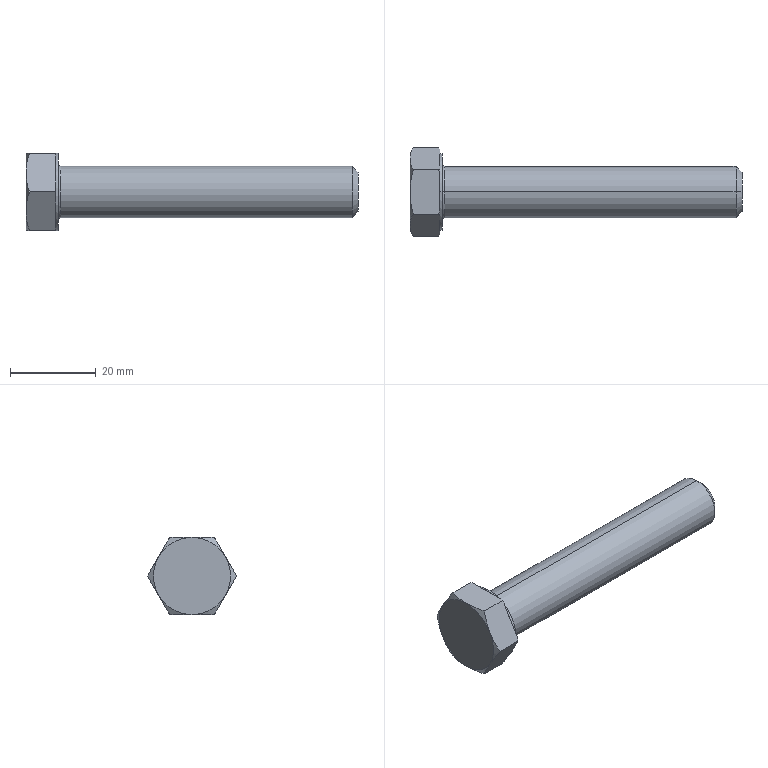Part | STEP file | 1 solid | 35 faces | box 77.5 x 20.785 x 18 mm | volume 9968 mm3 | plane 15 | cone 14 | cylinder 4 | spline 2 | commonest cylinder face diameters 12 x2 18 x2